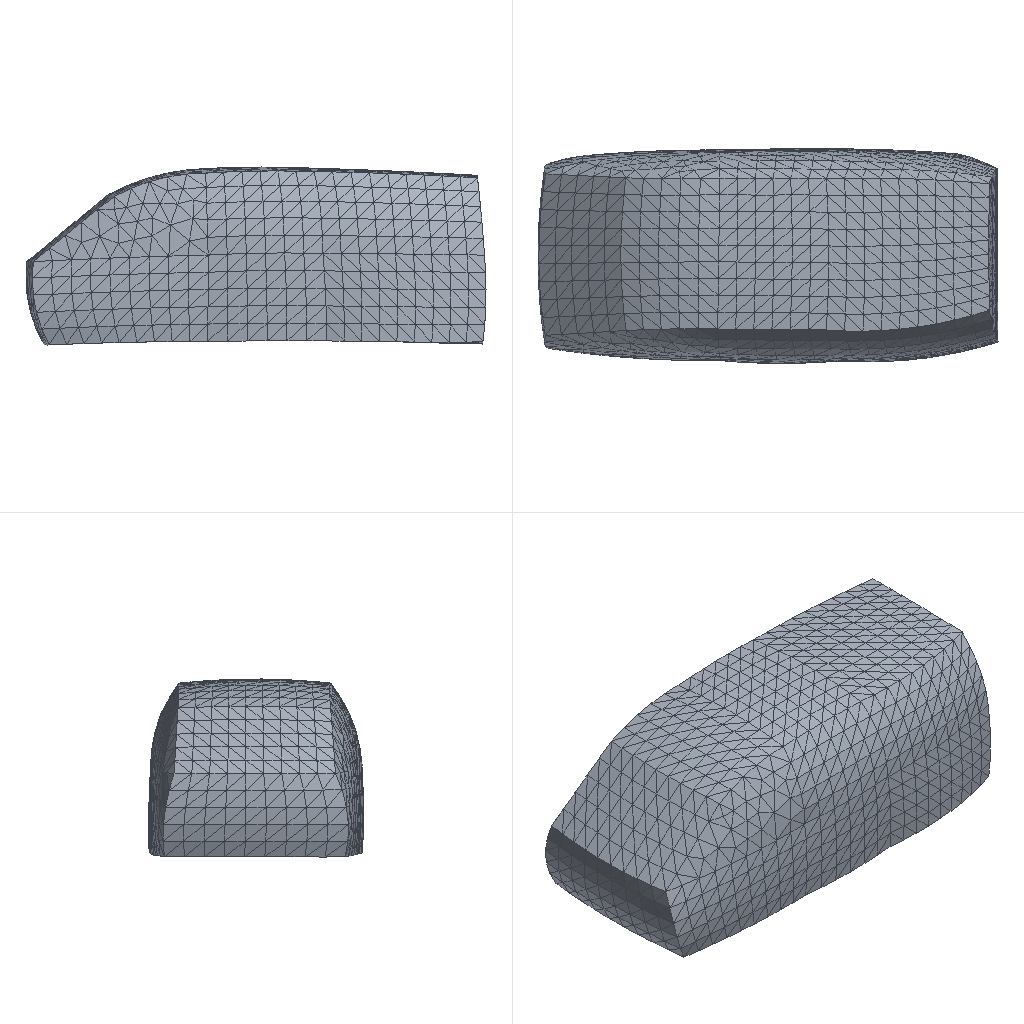Simulation study | abaqus
Set-up summary:
category,name,step,type,value,unit,region
solver,abaqus
solver,version,,,Abaqus/Standard 2020
units,not stated in the deck,,not stated
analysis,deck,,transient,transient
load_step,Step-1,Step-1,transient
load_step,requested,,,1
mesh,nodes,,,19168
mesh,elements,,,12810
element_type,C3D10,,solid,12810
load,load commands in deck,,count,6
bc,support commands in deck,,count,2
material,MATERIAL-1,,in results
check,setup vs results,,match,"per instance, exact: element labels, types and connectivity; labels of the nodes the elements use; coordinates of those nodes at SINGLE_PRECISION in 1 of 1 instance(s)"
Abaqus input file, long lists of numbers shortened:
*Heading
** Job name: Job-2 Model name: Model-2
** Generated by: Abaqus/CAE 2020
*Preprint, echo=NO, model=NO, history=NO, contact=NO
**
** PARTS
**
*Part, name=car2
*Node
      1,   2.277, -0.768,  0.6194
      2,   2.255,  0.7721,  0.6273
** (19166 more lines like these left out)
*Element, type=C3D10
    1,  1030,  1031,  1032,  1033,  2669,  2668,  2667,  2671,  2670,  2672
    2,  1030,  1031,  1034,  1035,  2669,  2674,  2673,  2676,  2675,  2677
** (12808 more lines like these left out)
*Nset, nset=Set-2, generate
     1,  19168,      1
*Elset, elset=Set-2, generate
     1,  12810,      1
*Nset, nset=Set-5, generate
     1,  19168,      1
*Elset, elset=Set-5, generate
     1,  12810,      1
** Section: Section-2
*Solid Section, elset=Set-5, material=Material-1
,
*End Part
**
**
** ASSEMBLY
**
*Assembly, name=Assembly
**
*Instance, name=car2-1, part=car2
*End Instance
**
*Node
      1,  0.1382,           0.,  0.8925
*Nset, nset=Set-1, instance=car2-1
     9,    10,    11,    12,    13,    14,    15,    16,    17,    18,    19,    20,    21,    22,    23,    24
    25,    98,    99,   100,   101,   102,   103,   104,   105,   106,   107,   108,   109,   110,   111,   112
** (81 more lines like these left out)
*Elset, elset=Set-1, instance=car2-1
    23,   114,  1038,  1114,  1529,  1617,  1626,  1648,  1651,  1738,  1745,  1753,  1757,  1765,  1788,  1797
  1800,  1805,  1811,  1819,  1873,  1879,  1880,  1974,  2043,  2067,  2230,  2259,  2321,  2379,  2417,  2552
** (36 more lines like these left out)
*Nset, nset=Set-4
 1,
*Nset, nset=m_Set-2
 1,
*Nset, nset=s_Set-2, instance=car2-1
     6,     7,    66,    67,    68,    69,    70,    71,    72,    73,    90,    91,    92,    93,    94,    95
    96,    97,   415,   416,   417,   418,   419,   420,   421,   422,   423,   424,   425,   426,   427,   428
** (10 more lines like these left out)
*Elset, elset=s_Set-2, instance=car2-1
   624,  2437,  2520,  2525,  2573,  2583,  2628,  2638,  2688,  2714,  2733,  2734,  2764,  2781,  2831,  2906
  2926,  2933,  2934,  2935,  2936,  2943,  2944,  2952,  2953,  2971,  2975,  2977,  2984,  2988,  2991,  2996
** (4 more lines like these left out)
*Elset, elset=_Surf-1_S3, internal, instance=car2-1
    37,   621,  1247,  1623,  1694,  1710,  1726,  1727,  1740,  1768,  1779,  1843,  1844,  1853,  1878,  1938
  1939,  1953,  1982,  2005,  2037,  2047,  2052,  2053,  2105,  2141,  2145,  2160,  2428,  2438,  2445,  2455
** (9 more lines like these left out)
*Elset, elset=_Surf-1_S1, internal, instance=car2-1
   206,  1838,  2488,  2490,  4087,  4143,  4217,  4230,  4244,  4276,  4277,  4335,  4338,  4442,  4636,  4671
  5139,  8313,  8388,  8421,  8651,  8907, 10148, 10385, 12244
*Elset, elset=_Surf-1_S2, internal, instance=car2-1
  2149,  2463,  2667,  2674,  3178,  3186,  4038,  4111,  4156,  4167,  4222,  4279,  4301,  4327,  4330,  4334
  4337,  4682,  4706,  4727,  4746,  4749,  4774,  6312,  6315,  6335,  6337,  6367,  6384,  7683, 10131
*Elset, elset=_Surf-1_S4, internal, instance=car2-1
   227,  2402,  2444,  3792,  3800,  4738,  4864,  7661,  8914,  9914, 10388
*Surface, type=ELEMENT, name=Surf-1
_Surf-1_S3, S3
_Surf-1_S1, S1
_Surf-1_S2, S2
_Surf-1_S4, S4
*Elset, elset=_Surf-2_S4, internal, instance=car2-1
  275, 2823, 3781, 5481, 7785
*Elset, elset=_Surf-2_S2, internal, instance=car2-1
  620, 2669, 2693, 2743, 2784, 2787, 2865, 3321, 3338, 3343, 3359, 3375, 3408, 3413, 3552, 3749
 5385,
*Elset, elset=_Surf-2_S3, internal, instance=car2-1
   651,  1538,  1746,  1867,  1913,  1948,  1961,  1968,  2021,  2086,  2137,  2173,  2323,  2340,  2634,  2718
  2761,  2774,  2835,  2860,  2892,  2893,  3198,  3217,  3237,  3241,  3308,  3332,  3336,  3339,  3344,  3350
** (11 more lines like these left out)
*Elset, elset=_Surf-2_S1, internal, instance=car2-1
  2279,  2695,  2804,  2891,  3264,  3285,  3296,  3323,  3342,  3351,  3368,  4290,  4452,  4586,  5371,  5664
 10081,
*Surface, type=ELEMENT, name=Surf-2
_Surf-2_S4, S4
_Surf-2_S2, S2
_Surf-2_S3, S3
_Surf-2_S1, S1
*Elset, elset=_Surf-3_S3, internal, instance=car2-1
   183,   244,   394,   402,   418,   462,   605,   711,  1380,  1658,  1792,  1809,  1870,  1875,  1898,  2668
  2737,  2905,  3628,  3661,  3763,  3770,  4012,  4037,  4060,  4069,  4100,  4179,  4307,  4384,  4436,  4717
** (19 more lines like these left out)
*Elset, elset=_Surf-3_S1, internal, instance=car2-1
  1096,  1789,  5099,  6614,  7004,  7390,  7574,  7576,  8743,  9783, 10339, 12099
*Elset, elset=_Surf-3_S2, internal, instance=car2-1
  4969,  5683,  6180,  6387,  6416,  6429,  6477,  6696,  6753,  6811,  7032,  7588,  8071, 11282
*Elset, elset=_Surf-3_S4, internal, instance=car2-1
  4695,  6589,  6637,  6698,  6706,  6834,  7137,  7160,  7466,  8594, 10905, 11159
*Surface, type=ELEMENT, name=Surf-3
_Surf-3_S3, S3
_Surf-3_S1, S1
_Surf-3_S2, S2
_Surf-3_S4, S4
*Elset, elset=_Surf-4_S4, internal, instance=car2-1
    66,    75,  1999,  4081,  7273, 10309, 12155
*Elset, elset=_Surf-4_S3, internal, instance=car2-1
  1304,  1993,  2078,  2122,  2126,  2157,  2168,  2177,  2201,  2322,  2332,  2337,  3497,  3528,  3533,  3546
  3555,  3564,  3567,  3608,  3715,  3804,  3812,  3819,  3829,  3832,  3836,  3845,  3849,  3850,  3856,  3866
** (3 more lines like these left out)
*Elset, elset=_Surf-4_S1, internal, instance=car2-1
 2250, 2271, 3498
*Elset, elset=_Surf-4_S2, internal, instance=car2-1
 3811, 3823, 3827
*Surface, type=ELEMENT, name=Surf-4
_Surf-4_S4, S4
_Surf-4_S3, S3
_Surf-4_S2, S2
_Surf-4_S1, S1
*Elset, elset=_Surf-5_S3, internal, instance=car2-1
    19,    43,   108,   113,   207,   321,   360,   401,  1280,  1616,  1620,  1636,  1642,  1646,  1657,  1660
  1663,  1666,  1667,  1684,  1695,  1701,  1707,  1717,  1718,  1720,  1721,  1722,  1736,  1737,  1750,  1752
** (23 more lines like these left out)
*Elset, elset=_Surf-5_S2, internal, instance=car2-1
  110, 2305, 2460, 2920, 3494, 4439, 4467, 4492, 4734, 5050, 5346
*Elset, elset=_Surf-5_S1, internal, instance=car2-1
 2149, 3193, 3403, 3800, 3836, 3932, 4441, 4468, 4493, 5369, 8239
*Elset, elset=_Surf-5_S4, internal, instance=car2-1
    96,  2120,  2199,  2204,  2302,  4641,  5439,  9193,  9399, 10072, 10656
*Surface, type=ELEMENT, name=Surf-5
_Surf-5_S3, S3
_Surf-5_S2, S2
_Surf-5_S4, S4
_Surf-5_S1, S1
*Surface, type=NODE, name=s_Set-2_CNS_, internal
s_Set-2, 1.
** Constraint: Constraint-1
*Coupling, constraint name=Constraint-1, ref node=m_Set-2, surface=s_Set-2_CNS_
*Kinematic
*End Assembly
*Amplitude, name=Amp-1, definition=PERIODIC
1,           1256.,              0.,              0.
           1.82,              0.
**
** MATERIALS
**
*Material, name=Material-1
*Density
7890.,
*Elastic
 2.1e+11, 0.3
**
** BOUNDARY CONDITIONS
**
** Name: BC-1 Type: 对称/反对称/完全固定
*Boundary
Set-1, ENCASTRE
** ----------------------------------------------------------------
**
** STEP: Step-1
**
*Step, name=Step-1, nlgeom=YES, inc=1000
*Dynamic
0.001,0.1,1e-06
**
** BOUNDARY CONDITIONS
**
** Name: BC-2 Type: 速度/角速度
*Boundary, amplitude=Amp-1, type=VELOCITY
Set-4, 1, 1, 1.
**
** LOADS
**
** Name: Load-1   Type: Pressure
*Dsload
Surf-1, P, 0.117
** Name: Load-2   Type: Pressure
*Dsload
Surf-2, P, 0.117
** Name: Load-3   Type: Pressure
*Dsload
Surf-3, P, 0.117
** Name: Load-4   Type: Pressure
*Dsload
Surf-4, P, 0.117
** Name: Load-5   Type: Pressure
*Dsload
Surf-5, P, 0.117
**
** OUTPUT REQUESTS
**
*Restart, write, frequency=0
**
** FIELD OUTPUT: F-Output-1
**
*Output, field, frequency=1
*Node Output
A, CF, RF, U, V
*Element Output, directions=YES
E, LE, MISES, P, PE, PEEQ, PEMAG, S, SF
*Contact Output
CDISP, CSTRESS
**
** HISTORY OUTPUT: H-Output-1
**
*Output, history, variable=PRESELECT
*End Step
Results summary:
result,step,,partial,increments=83 time=0.0186/0.1
result,analysis,,,transient
result,last_loadstep,,,1
result,primary field,,,U
result,reaction total,,FX,20102953.326,model units
result,reaction total,,FY,-360968.573,model units
result,reaction total,,FZ,13410527.194,model units